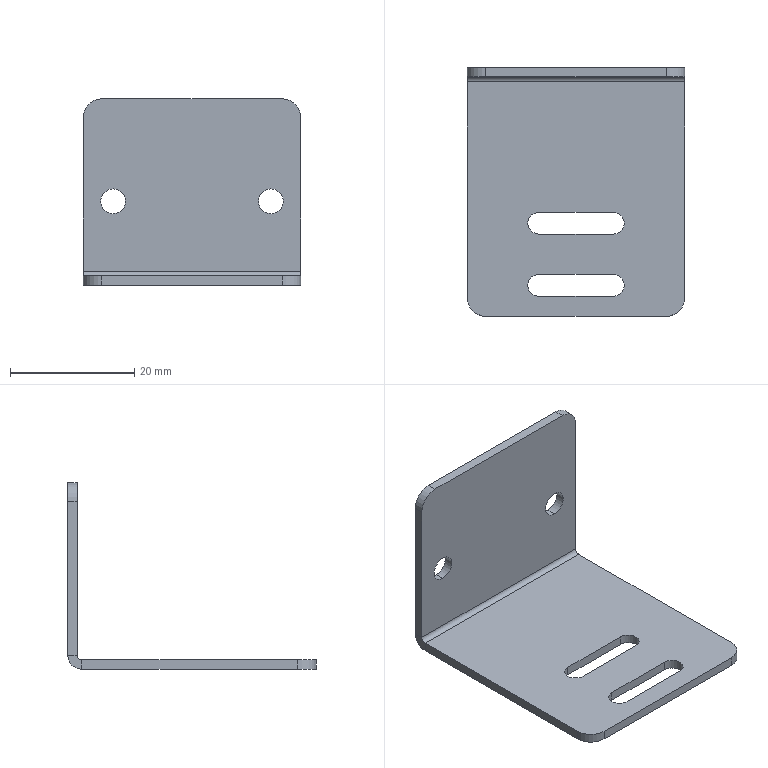Part | STEP file | PN_0039(Default) | 1 solid | 32 faces | box 35 x 40 x 30 mm | volume 3359 mm3 | cylinder 16 | plane 16 | commonest cylinder face diameters 3.5 x6 4 x4 6 x4 1.473 x1 4.473 x1